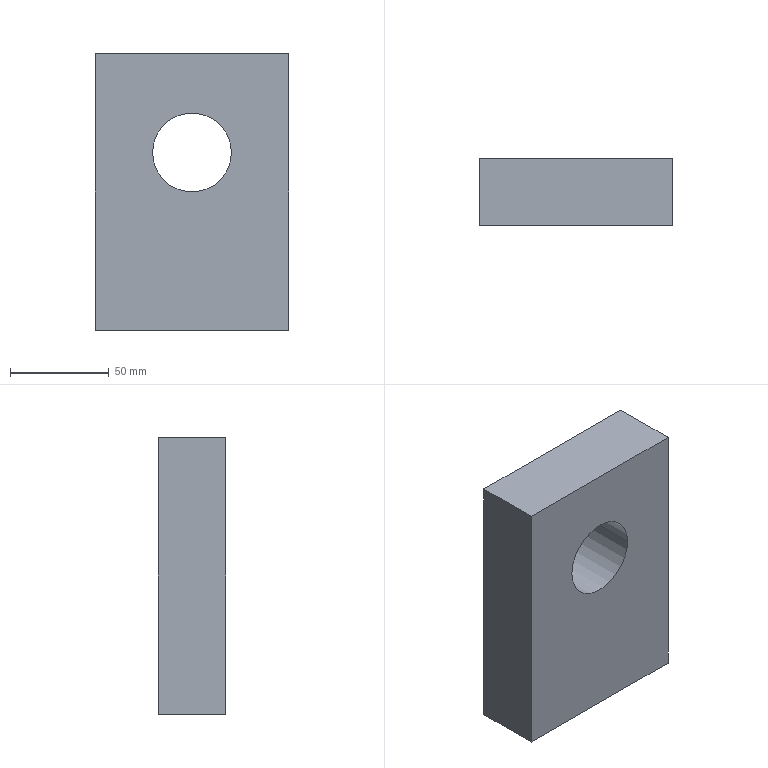Part | STEP file | PN_0012 connecting plate | 1 solid | 72 faces | box 98 x 34 x 140 mm | volume 419089 mm3 | cylinder 34 | cone 32 | plane 6 | commonest cylinder face diameters 4.2 x16 6.8 x8 3.3 x4 5 x4 40 x2